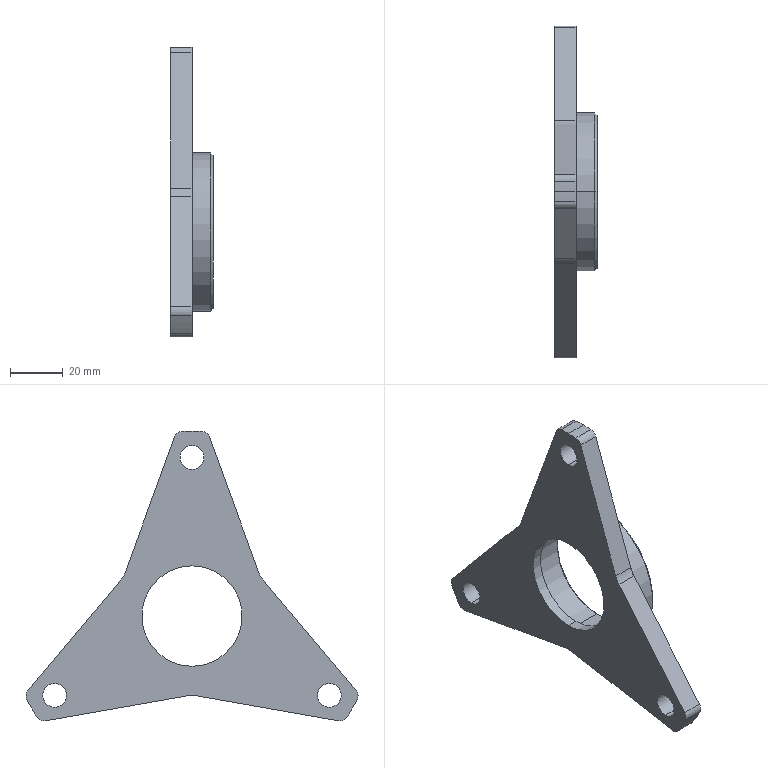Part | SolidWorks | features BaseBody 1 | 1 solid | 41 faces | box 16 x 125.605 x 109.685 mm | volume 50811 mm3 | cylinder 25 | plane 12 | cone 4 | commonest cylinder face diameters 6 x6 9 x6 140 x4 20 x3 38 x2 42 x2
STEP:
#1=CARTESIAN_POINT('',(8.,-51.962,-34.5));
#2=VERTEX_POINT('',#1);
#3=CARTESIAN_POINT('',(8.,-51.962,-25.5));
#4=VERTEX_POINT('',#3);
#5=CARTESIAN_POINT('',(8.,-51.962,-30.));
#6=DIRECTION('',(-1.,0.,0.));
#7=DIRECTION('',(0.,0.,1.));
#8=AXIS2_PLACEMENT_3D('',#5,#6,#7);
#9=CIRCLE('',#8,4.5);
#10=EDGE_CURVE('',#2,#4,#9,.T.);
#11=ORIENTED_EDGE('',*,*,#10,.F.);
#12=CARTESIAN_POINT('',(0.,-51.962,-34.5));
#13=VERTEX_POINT('',#12);
#14=CARTESIAN_POINT('',(0.,-51.962,-34.5));
#15=DIRECTION('',(-1.,0.,0.));
#16=VECTOR('',#15,1000.);
#17=LINE('',#14,#16);
#18=EDGE_CURVE('',#2,#13,#17,.T.);
#19=ORIENTED_EDGE('',*,*,#18,.T.);
#20=CARTESIAN_POINT('',(0.,-51.962,-25.5));
#21=VERTEX_POINT('',#20);
#22=CARTESIAN_POINT('',(0.,-51.962,-30.));
#23=DIRECTION('',(-1.,0.,0.));
#24=DIRECTION('',(0.,0.,1.));
#25=AXIS2_PLACEMENT_3D('',#22,#23,#24);
#26=CIRCLE('',#25,4.5);
#27=EDGE_CURVE('',#13,#21,#26,.T.);
#28=ORIENTED_EDGE('',*,*,#27,.T.);
#29=CARTESIAN_POINT('',(0.,-51.962,-25.5));
#30=DIRECTION('',(-1.,0.,0.));
#31=VECTOR('',#30,1000.);
#32=LINE('',#29,#31);
#33=EDGE_CURVE('',#4,#21,#32,.T.);
#34=ORIENTED_EDGE('',*,*,#33,.F.);
#35=EDGE_LOOP('',(#11,#19,#28,#34));
#36=FACE_OUTER_BOUND('',#35,.T.);
#37=CARTESIAN_POINT('',(0.,-51.962,-30.));
#38=DIRECTION('',(-1.,0.,0.));
#39=DIRECTION('',(0.,0.,1.));
#40=AXIS2_PLACEMENT_3D('',#37,#38,#39);
#41=CYLINDRICAL_SURFACE('',#40,4.5);
#42=ADVANCED_FACE('',(#36),#41,.F.);
#43=CARTESIAN_POINT('',(8.,-3.905,69.891));
#44=VERTEX_POINT('',#43);
#45=CARTESIAN_POINT('',(8.,0.,70.));
#46=VERTEX_POINT('',#45);
#47=CARTESIAN_POINT('',(8.,0.,0.));
#48=DIRECTION('',(-1.,0.,0.));
#49=DIRECTION('',(0.,0.,1.));
#50=AXIS2_PLACEMENT_3D('',#47,#48,#49);
#51=CIRCLE('',#50,70.);
#52=EDGE_CURVE('',#44,#46,#51,.T.);
#53=ORIENTED_EDGE('',*,*,#52,.T.);
#54=CARTESIAN_POINT('',(0.,0.,70.));
#55=VERTEX_POINT('',#54);
#56=CARTESIAN_POINT('',(0.,0.,70.));
#57=DIRECTION('',(-1.,0.,0.));
#58=VECTOR('',#57,1000.);
#59=LINE('',#56,#58);
#60=EDGE_CURVE('',#46,#55,#59,.T.);
#61=ORIENTED_EDGE('',*,*,#60,.T.);
#62=CARTESIAN_POINT('',(0.,-3.905,69.891));
#63=VERTEX_POINT('',#62);
#64=CARTESIAN_POINT('',(0.,0.,0.));
#65=DIRECTION('',(1.,0.,0.));
#66=DIRECTION('',(0.,0.,1.));
#67=AXIS2_PLACEMENT_3D('',#64,#65,#66);
#68=CIRCLE('',#67,70.);
#69=EDGE_CURVE('',#55,#63,#68,.T.);
#70=ORIENTED_EDGE('',*,*,#69,.T.);
#71=CARTESIAN_POINT('',(0.,-3.905,69.891));
#72=DIRECTION('',(-1.,0.,0.));
#73=VECTOR('',#72,1000.);
#74=LINE('',#71,#73);
#75=EDGE_CURVE('',#44,#63,#74,.T.);
#76=ORIENTED_EDGE('',*,*,#75,.F.);
#77=EDGE_LOOP('',(#53,#61,#70,#76));
#78=FACE_OUTER_BOUND('',#77,.T.);
#79=CARTESIAN_POINT('',(0.,0.,0.));
#80=DIRECTION('',(-1.,0.,0.));
#81=DIRECTION('',(0.,0.,1.));
#82=AXIS2_PLACEMENT_3D('',#79,#80,#81);
#83=CYLINDRICAL_SURFACE('',#82,70.);
#84=ADVANCED_FACE('',(#78),#83,.T.);
#85=CARTESIAN_POINT('',(4.,0.,-19.));
#86=VERTEX_POINT('',#85);
#87=CARTESIAN_POINT('',(4.,0.,19.));
#88=VERTEX_POINT('',#87);
#89=CARTESIAN_POINT('',(4.,0.,0.));
#90=DIRECTION('',(-1.,0.,0.));
#91=DIRECTION('',(0.,0.,1.));
#92=AXIS2_PLACEMENT_3D('',#89,#90,#91);
#93=CIRCLE('',#92,19.);
#94=EDGE_CURVE('',#86,#88,#93,.T.);
#95=ORIENTED_EDGE('',*,*,#94,.F.);
#96=CARTESIAN_POINT('',(0.,0.,-19.));
#97=VERTEX_POINT('',#96);
#98=CARTESIAN_POINT('',(0.,0.,-19.));
#99=DIRECTION('',(-1.,0.,0.));
#100=VECTOR('',#99,1000.);
#101=LINE('',#98,#100);
#102=EDGE_CURVE('',#86,#97,#101,.T.);
#103=ORIENTED_EDGE('',*,*,#102,.T.);
#104=CARTESIAN_POINT('',(0.,0.,19.));
#105=VERTEX_POINT('',#104);
#106=CARTESIAN_POINT('',(0.,0.,0.));
#107=DIRECTION('',(-1.,0.,0.));
#108=DIRECTION('',(0.,0.,1.));
#109=AXIS2_PLACEMENT_3D('',#106,#107,#108);
#110=CIRCLE('',#109,19.);
#111=EDGE_CURVE('',#97,#105,#110,.T.);
#112=ORIENTED_EDGE('',*,*,#111,.T.);
#113=CARTESIAN_POINT('',(0.,0.,19.));
#114=DIRECTION('',(-1.,0.,0.));
#115=VECTOR('',#114,1000.);
#116=LINE('',#113,#115);
#117=EDGE_CURVE('',#88,#105,#116,.T.);
#118=ORIENTED_EDGE('',*,*,#117,.F.);
#119=EDGE_LOOP('',(#95,#103,#112,#118));
#120=FACE_OUTER_BOUND('',#119,.T.);
#121=CARTESIAN_POINT('',(0.,0.,0.));
#122=DIRECTION('',(-1.,0.,0.));
#123=DIRECTION('',(0.,0.,1.));
#124=AXIS2_PLACEMENT_3D('',#121,#122,#123);
#125=CYLINDRICAL_SURFACE('',#124,19.);
#126=ADVANCED_FACE('',(#120),#125,.F.);
#127=CARTESIAN_POINT('',(8.,0.,55.5));
#128=VERTEX_POINT('',#127);
#129=CARTESIAN_POINT('',(8.,0.,64.5));
#130=VERTEX_POINT('',#129);
#131=CARTESIAN_POINT('',(8.,0.,60.));
#132=DIRECTION('',(-1.,0.,0.));
#133=DIRECTION('',(0.,0.,1.));
#134=AXIS2_PLACEMENT_3D('',#131,#132,#133);
#135=CIRCLE('',#134,4.5);
#136=EDGE_CURVE('',#128,#130,#135,.T.);
#137=ORIENTED_EDGE('',*,*,#136,.F.);
#138=CARTESIAN_POINT('',(0.,0.,55.5));
#139=VERTEX_POINT('',#138);
#140=CARTESIAN_POINT('',(0.,0.,55.5));
#141=DIRECTION('',(-1.,0.,0.));
#142=VECTOR('',#141,1000.);
#143=LINE('',#140,#142);
#144=EDGE_CURVE('',#128,#139,#143,.T.);
#145=ORIENTED_EDGE('',*,*,#144,.T.);
#146=CARTESIAN_POINT('',(0.,0.,64.5));
#147=VERTEX_POINT('',#146);
#148=CARTESIAN_POINT('',(0.,0.,60.));
#149=DIRECTION('',(-1.,0.,0.));
#150=DIRECTION('',(0.,0.,1.));
#151=AXIS2_PLACEMENT_3D('',#148,#149,#150);
#152=CIRCLE('',#151,4.5);
#153=EDGE_CURVE('',#139,#147,#152,.T.);
#154=ORIENTED_EDGE('',*,*,#153,.T.);
#155=CARTESIAN_POINT('',(0.,0.,64.5));
#156=DIRECTION('',(-1.,0.,0.));
#157=VECTOR('',#156,1000.);
#158=LINE('',#155,#157);
#159=EDGE_CURVE('',#130,#147,#158,.T.);
#160=ORIENTED_EDGE('',*,*,#159,.F.);
#161=EDGE_LOOP('',(#137,#145,#154,#160));
#162=FACE_OUTER_BOUND('',#161,.T.);
#163=CARTESIAN_POINT('',(0.,0.,60.));
#164=DIRECTION('',(-1.,0.,0.));
#165=DIRECTION('',(0.,0.,1.));
#166=AXIS2_PLACEMENT_3D('',#163,#164,#165);
#167=CYLINDRICAL_SURFACE('',#166,4.5);
#168=ADVANCED_FACE('',(#162),#167,.F.);
#169=CARTESIAN_POINT('',(8.,51.962,-34.5));
#170=VERTEX_POINT('',#169);
#171=CARTESIAN_POINT('',(8.,51.962,-25.5));
#172=VERTEX_POINT('',#171);
#173=CARTESIAN_POINT('',(8.,51.962,-30.));
#174=DIRECTION('',(-1.,0.,0.));
#175=DIRECTION('',(0.,0.,1.));
#176=AXIS2_PLACEMENT_3D('',#173,#174,#175);
#177=CIRCLE('',#176,4.5);
#178=EDGE_CURVE('',#170,#172,#177,.T.);
#179=ORIENTED_EDGE('',*,*,#178,.F.);
#180=CARTESIAN_POINT('',(0.,51.962,-34.5));
#181=VERTEX_POINT('',#180);
#182=CARTESIAN_POINT('',(0.,51.962,-34.5));
#183=DIRECTION('',(-1.,0.,0.));
#184=VECTOR('',#183,1000.);
#185=LINE('',#182,#184);
#186=EDGE_CURVE('',#170,#181,#185,.T.);
#187=ORIENTED_EDGE('',*,*,#186,.T.);
#188=CARTESIAN_POINT('',(0.,51.962,-25.5));
#189=VERTEX_POINT('',#188);
#190=CARTESIAN_POINT('',(0.,51.962,-30.));
#191=DIRECTION('',(-1.,0.,0.));
#192=DIRECTION('',(0.,0.,1.));
#193=AXIS2_PLACEMENT_3D('',#190,#191,#192);
#194=CIRCLE('',#193,4.5);
#195=EDGE_CURVE('',#181,#189,#194,.T.);
#196=ORIENTED_EDGE('',*,*,#195,.T.);
#197=CARTESIAN_POINT('',(0.,51.962,-25.5));
#198=DIRECTION('',(-1.,0.,0.));
#199=VECTOR('',#198,1000.);
#200=LINE('',#197,#199);
#201=EDGE_CURVE('',#172,#189,#200,.T.);
#202=ORIENTED_EDGE('',*,*,#201,.F.);
#203=EDGE_LOOP('',(#179,#187,#196,#202));
#204=FACE_OUTER_BOUND('',#203,.T.);
#205=CARTESIAN_POINT('',(0.,51.962,-30.));
#206=DIRECTION('',(-1.,0.,0.));
#207=DIRECTION('',(0.,0.,1.));
#208=AXIS2_PLACEMENT_3D('',#205,#206,#207);
#209=CYLINDRICAL_SURFACE('',#208,4.5);
#210=ADVANCED_FACE('',(#204),#209,.F.);
#211=CARTESIAN_POINT('',(15.,0.,30.));
#212=VERTEX_POINT('',#211);
#213=CARTESIAN_POINT('',(15.,0.,-30.));
#214=VERTEX_POINT('',#213);
#215=CARTESIAN_POINT('',(15.,0.,0.));
#216=DIRECTION('',(-1.,0.,0.));
#217=DIRECTION('',(0.,0.,1.));
#218=AXIS2_PLACEMENT_3D('',#215,#216,#217);
#219=CIRCLE('',#218,30.);
#220=EDGE_CURVE('',#212,#214,#219,.T.);
#221=ORIENTED_EDGE('',*,*,#220,.T.);
#222=CARTESIAN_POINT('',(8.,0.,-30.));
#223=VERTEX_POINT('',#222);
#224=CARTESIAN_POINT('',(0.,0.,-30.));
#225=DIRECTION('',(-1.,0.,0.));
#226=VECTOR('',#225,1000.);
#227=LINE('',#224,#226);
#228=EDGE_CURVE('',#214,#223,#227,.T.);
#229=ORIENTED_EDGE('',*,*,#228,.T.);
#230=CARTESIAN_POINT('',(8.,25.981,15.));
#231=VERTEX_POINT('',#230);
#232=CARTESIAN_POINT('',(8.,0.,0.));
#233=DIRECTION('',(1.,0.,0.));
#234=DIRECTION('',(0.,0.,1.));
#235=AXIS2_PLACEMENT_3D('',#232,#233,#234);
#236=CIRCLE('',#235,30.);
#237=EDGE_CURVE('',#223,#231,#236,.T.);
#238=ORIENTED_EDGE('',*,*,#237,.T.);
#239=CARTESIAN_POINT('',(8.,0.,30.));
#240=VERTEX_POINT('',#239);
#241=CARTESIAN_POINT('',(8.,0.,0.));
#242=DIRECTION('',(1.,0.,0.));
#243=DIRECTION('',(0.,0.,1.));
#244=AXIS2_PLACEMENT_3D('',#241,#242,#243);
#245=CIRCLE('',#244,30.);
#246=EDGE_CURVE('',#231,#240,#245,.T.);
#247=ORIENTED_EDGE('',*,*,#246,.T.);
#248=CARTESIAN_POINT('',(0.,0.,30.));
#249=DIRECTION('',(-1.,0.,0.));
#250=VECTOR('',#249,1000.);
#251=LINE('',#248,#250);
#252=EDGE_CURVE('',#212,#240,#251,.T.);
#253=ORIENTED_EDGE('',*,*,#252,.F.);
#254=EDGE_LOOP('',(#221,#229,#238,#247,#253));
#255=FACE_OUTER_BOUND('',#254,.T.);
#256=CARTESIAN_POINT('',(0.,0.,0.));
#257=DIRECTION('',(-1.,0.,0.));
#258=DIRECTION('',(0.,0.,1.));
#259=AXIS2_PLACEMENT_3D('',#256,#257,#258);
#260=CYLINDRICAL_SURFACE('',#259,30.);
#261=ADVANCED_FACE('',(#255),#260,.T.);
#262=CARTESIAN_POINT('',(15.,0.,-21.));
#263=VERTEX_POINT('',#262);
#264=CARTESIAN_POINT('',(15.,0.,21.));
#265=VERTEX_POINT('',#264);
#266=CARTESIAN_POINT('',(15.,0.,0.));
#267=DIRECTION('',(-1.,0.,0.));
#268=DIRECTION('',(0.,0.,1.));
#269=AXIS2_PLACEMENT_3D('',#266,#267,#268);
#270=CIRCLE('',#269,21.);
#271=EDGE_CURVE('',#263,#265,#270,.T.);
#272=ORIENTED_EDGE('',*,*,#271,.F.);
#273=CARTESIAN_POINT('',(4.,0.,-21.));
#274=VERTEX_POINT('',#273);
#275=CARTESIAN_POINT('',(0.,0.,-21.));
#276=DIRECTION('',(-1.,0.,0.));
#277=VECTOR('',#276,1000.);
#278=LINE('',#275,#277);
#279=EDGE_CURVE('',#263,#274,#278,.T.);
#280=ORIENTED_EDGE('',*,*,#279,.T.);
#281=CARTESIAN_POINT('',(4.,0.,21.));
#282=VERTEX_POINT('',#281);
#283=CARTESIAN_POINT('',(4.,0.,0.));
#284=DIRECTION('',(-1.,0.,0.));
#285=DIRECTION('',(0.,0.,1.));
#286=AXIS2_PLACEMENT_3D('',#283,#284,#285);
#287=CIRCLE('',#286,21.);
#288=EDGE_CURVE('',#274,#282,#287,.T.);
#289=ORIENTED_EDGE('',*,*,#288,.T.);
#290=CARTESIAN_POINT('',(0.,0.,21.));
#291=DIRECTION('',(-1.,0.,0.));
#292=VECTOR('',#291,1000.);
#293=LINE('',#290,#292);
#294=EDGE_CURVE('',#265,#282,#293,.T.);
#295=ORIENTED_EDGE('',*,*,#294,.F.);
#296=EDGE_LOOP('',(#272,#280,#289,#295));
#297=FACE_OUTER_BOUND('',#296,.T.);
#298=CARTESIAN_POINT('',(0.,0.,0.));
#299=DIRECTION('',(-1.,0.,0.));
#300=DIRECTION('',(0.,0.,1.));
#301=AXIS2_PLACEMENT_3D('',#298,#299,#300);
#302=CYLINDRICAL_SURFACE('',#301,21.);
#303=ADVANCED_FACE('',(#297),#302,.F.);
#304=CARTESIAN_POINT('',(16.,0.,29.));
#305=VERTEX_POINT('',#304);
#306=CARTESIAN_POINT('',(16.,0.,-29.));
#307=VERTEX_POINT('',#306);
#308=CARTESIAN_POINT('',(16.,0.,0.));
#309=DIRECTION('',(-1.,0.,0.));
#310=DIRECTION('',(0.,0.,1.));
#311=AXIS2_PLACEMENT_3D('',#308,#309,#310);
#312=CIRCLE('',#311,29.);
#313=EDGE_CURVE('',#305,#307,#312,.T.);
#314=ORIENTED_EDGE('',*,*,#313,.T.);
#315=CARTESIAN_POINT('',(15.,0.,-30.));
#316=DIRECTION('',(-0.7071,0.,-0.7071));
#317=VECTOR('',#316,1000.);
#318=LINE('',#315,#317);
#319=EDGE_CURVE('',#307,#214,#318,.T.);
#320=ORIENTED_EDGE('',*,*,#319,.T.);
#321=ORIENTED_EDGE('',*,*,#220,.F.);
#322=CARTESIAN_POINT('',(15.,0.,30.));
#323=DIRECTION('',(-0.7071,0.,0.7071));
#324=VECTOR('',#323,1000.);
#325=LINE('',#322,#324);
#326=EDGE_CURVE('',#305,#212,#325,.T.);
#327=ORIENTED_EDGE('',*,*,#326,.F.);
#328=EDGE_LOOP('',(#314,#320,#321,#327));
#329=FACE_OUTER_BOUND('',#328,.T.);
#330=CARTESIAN_POINT('',(15.,0.,0.));
#331=DIRECTION('',(-1.,0.,0.));
#332=DIRECTION('',(0.,0.,1.));
#333=AXIS2_PLACEMENT_3D('',#330,#331,#332);
#334=CONICAL_SURFACE('',#333,30.,0.7854);
#335=ADVANCED_FACE('',(#329),#334,.T.);
#336=ORIENTED_EDGE('',*,*,#271,.T.);
#337=CARTESIAN_POINT('',(16.,0.,22.));
#338=VERTEX_POINT('',#337);
#339=CARTESIAN_POINT('',(16.,0.,22.));
#340=DIRECTION('',(0.7071,0.,0.7071));
#341=VECTOR('',#340,1000.);
#342=LINE('',#339,#341);
#343=EDGE_CURVE('',#265,#338,#342,.T.);
#344=ORIENTED_EDGE('',*,*,#343,.T.);
#345=CARTESIAN_POINT('',(16.,0.,-22.));
#346=VERTEX_POINT('',#345);
#347=CARTESIAN_POINT('',(16.,0.,0.));
#348=DIRECTION('',(-1.,0.,0.));
#349=DIRECTION('',(0.,0.,-1.));
#350=AXIS2_PLACEMENT_3D('',#347,#348,#349);
#351=CIRCLE('',#350,22.);
#352=EDGE_CURVE('',#346,#338,#351,.T.);
#353=ORIENTED_EDGE('',*,*,#352,.F.);
#354=CARTESIAN_POINT('',(16.,0.,-22.));
#355=DIRECTION('',(0.7071,0.,-0.7071));
#356=VECTOR('',#355,1000.);
#357=LINE('',#354,#356);
#358=EDGE_CURVE('',#263,#346,#357,.T.);
#359=ORIENTED_EDGE('',*,*,#358,.F.);
#360=EDGE_LOOP('',(#336,#344,#353,#359));
#361=FACE_OUTER_BOUND('',#360,.T.);
#362=CARTESIAN_POINT('',(16.,0.,0.));
#363=DIRECTION('',(1.,0.,0.));
#364=DIRECTION('',(0.,0.,-1.));
#365=AXIS2_PLACEMENT_3D('',#362,#363,#364);
#366=CONICAL_SURFACE('',#365,22.,0.7854);
#367=ADVANCED_FACE('',(#361),#366,.F.);
#368=CARTESIAN_POINT('',(0.,-51.962,-30.));
#369=DIRECTION('',(-1.,0.,0.));
#370=DIRECTION('',(0.,0.,1.));
#371=AXIS2_PLACEMENT_3D('',#368,#369,#370);
#372=CIRCLE('',#371,4.5);
#373=EDGE_CURVE('',#21,#13,#372,.T.);
#374=ORIENTED_EDGE('',*,*,#373,.F.);
#375=ORIENTED_EDGE('',*,*,#27,.F.);
#376=EDGE_LOOP('',(#374,#375));
#377=FACE_BOUND('',#376,.T.);
#378=CARTESIAN_POINT('',(0.,-58.575,-38.328));
#379=VERTEX_POINT('',#378);
#380=CARTESIAN_POINT('',(0.,-55.543,-39.64));
#381=VERTEX_POINT('',#380);
#382=CARTESIAN_POINT('',(0.,-56.064,-36.685));
#383=DIRECTION('',(1.,0.,0.));
#384=DIRECTION('',(0.,0.,1.));
#385=AXIS2_PLACEMENT_3D('',#382,#383,#384);
#386=CIRCLE('',#385,3.);
#387=EDGE_CURVE('',#379,#381,#386,.T.);
#388=ORIENTED_EDGE('',*,*,#387,.F.);
#389=CARTESIAN_POINT('',(0.,-62.48,-31.563));
#390=VERTEX_POINT('',#389);
#391=CARTESIAN_POINT('',(0.,0.,0.));
#392=DIRECTION('',(1.,0.,0.));
#393=DIRECTION('',(0.,0.,1.));
#394=AXIS2_PLACEMENT_3D('',#391,#392,#393);
#395=CIRCLE('',#394,70.);
#396=EDGE_CURVE('',#390,#379,#395,.T.);
#397=ORIENTED_EDGE('',*,*,#396,.F.);
#398=CARTESIAN_POINT('',(0.,-62.101,-28.282));
#399=VERTEX_POINT('',#398);
#400=CARTESIAN_POINT('',(0.,-59.802,-30.211));
#401=DIRECTION('',(1.,0.,0.));
#402=DIRECTION('',(0.,0.,1.));
#403=AXIS2_PLACEMENT_3D('',#400,#401,#402);
#404=CIRCLE('',#403,3.);
#405=EDGE_CURVE('',#399,#390,#404,.T.);
#406=ORIENTED_EDGE('',*,*,#405,.F.);
#407=CARTESIAN_POINT('',(0.,-26.981,13.572));
#408=VERTEX_POINT('',#407);
#409=CARTESIAN_POINT('',(0.,-26.981,13.572));
#410=DIRECTION('',(0.,-0.6428,-0.766));
#411=VECTOR('',#410,1000.);
#412=LINE('',#409,#411);
#413=EDGE_CURVE('',#408,#399,#412,.T.);
#414=ORIENTED_EDGE('',*,*,#413,.F.);
#415=CARTESIAN_POINT('',(0.,-25.244,16.58));
#416=VERTEX_POINT('',#415);
#417=CARTESIAN_POINT('',(0.,-34.641,20.));
#418=DIRECTION('',(-1.,0.,0.));
#419=DIRECTION('',(0.,0.,-1.));
#420=AXIS2_PLACEMENT_3D('',#417,#418,#419);
#421=CIRCLE('',#420,10.);
#422=EDGE_CURVE('',#416,#408,#421,.T.);
#423=ORIENTED_EDGE('',*,*,#422,.F.);
#424=CARTESIAN_POINT('',(0.,-6.557,67.922));
#425=VERTEX_POINT('',#424);
#426=CARTESIAN_POINT('',(0.,-6.557,67.922));
#427=DIRECTION('',(0.,-0.342,-0.9397));
#428=VECTOR('',#427,1000.);
#429=LINE('',#426,#428);
#430=EDGE_CURVE('',#425,#416,#429,.T.);
#431=ORIENTED_EDGE('',*,*,#430,.F.);
#432=CARTESIAN_POINT('',(0.,-3.738,66.896));
#433=DIRECTION('',(1.,0.,0.));
#434=DIRECTION('',(0.,0.,1.));
#435=AXIS2_PLACEMENT_3D('',#432,#433,#434);
#436=CIRCLE('',#435,3.);
#437=EDGE_CURVE('',#63,#425,#436,.T.);
#438=ORIENTED_EDGE('',*,*,#437,.F.);
#439=ORIENTED_EDGE('',*,*,#69,.F.);
#440=CARTESIAN_POINT('',(0.,3.905,69.891));
#441=VERTEX_POINT('',#440);
#442=CARTESIAN_POINT('',(0.,0.,0.));
#443=DIRECTION('',(1.,0.,0.));
#444=DIRECTION('',(0.,0.,1.));
#445=AXIS2_PLACEMENT_3D('',#442,#443,#444);
#446=CIRCLE('',#445,70.);
#447=EDGE_CURVE('',#441,#55,#446,.T.);
#448=ORIENTED_EDGE('',*,*,#447,.F.);
#449=CARTESIAN_POINT('',(0.,6.557,67.922));
#450=VERTEX_POINT('',#449);
#451=CARTESIAN_POINT('',(0.,3.738,66.896));
#452=DIRECTION('',(1.,0.,0.));
#453=DIRECTION('',(0.,0.,1.));
#454=AXIS2_PLACEMENT_3D('',#451,#452,#453);
#455=CIRCLE('',#454,3.);
#456=EDGE_CURVE('',#450,#441,#455,.T.);
#457=ORIENTED_EDGE('',*,*,#456,.F.);
#458=CARTESIAN_POINT('',(0.,25.244,16.58));
#459=VERTEX_POINT('',#458);
#460=CARTESIAN_POINT('',(0.,25.244,16.58));
#461=DIRECTION('',(0.,-0.342,0.9397));
#462=VECTOR('',#461,1000.);
#463=LINE('',#460,#462);
#464=EDGE_CURVE('',#459,#450,#463,.T.);
#465=ORIENTED_EDGE('',*,*,#464,.F.);
#466=CARTESIAN_POINT('',(0.,26.981,13.572));
#467=VERTEX_POINT('',#466);
#468=CARTESIAN_POINT('',(0.,34.641,20.));
#469=DIRECTION('',(-1.,0.,0.));
#470=DIRECTION('',(0.,0.,-1.));
#471=AXIS2_PLACEMENT_3D('',#468,#469,#470);
#472=CIRCLE('',#471,10.);
#473=EDGE_CURVE('',#467,#459,#472,.T.);
#474=ORIENTED_EDGE('',*,*,#473,.F.);
#475=CARTESIAN_POINT('',(0.,62.101,-28.282));
#476=VERTEX_POINT('',#475);
#477=CARTESIAN_POINT('',(0.,62.101,-28.282));
#478=DIRECTION('',(0.,-0.6428,0.766));
#479=VECTOR('',#478,1000.);
#480=LINE('',#477,#479);
#481=EDGE_CURVE('',#476,#467,#480,.T.);
#482=ORIENTED_EDGE('',*,*,#481,.F.);
#483=CARTESIAN_POINT('',(0.,62.48,-31.563));
#484=VERTEX_POINT('',#483);
#485=CARTESIAN_POINT('',(0.,59.802,-30.211));
#486=DIRECTION('',(1.,0.,0.));
#487=DIRECTION('',(0.,0.,1.));
#488=AXIS2_PLACEMENT_3D('',#485,#486,#487);
#489=CIRCLE('',#488,3.);
#490=EDGE_CURVE('',#484,#476,#489,.T.);
#491=ORIENTED_EDGE('',*,*,#490,.F.);
#492=CARTESIAN_POINT('',(0.,58.575,-38.328));
#493=VERTEX_POINT('',#492);
#494=CARTESIAN_POINT('',(0.,0.,0.));
#495=DIRECTION('',(1.,0.,0.));
#496=DIRECTION('',(0.,0.,1.));
#497=AXIS2_PLACEMENT_3D('',#494,#495,#496);
#498=CIRCLE('',#497,70.);
#499=EDGE_CURVE('',#493,#484,#498,.T.);
#500=ORIENTED_EDGE('',*,*,#499,.F.);
#501=CARTESIAN_POINT('',(0.,55.543,-39.64));
#502=VERTEX_POINT('',#501);
#503=CARTESIAN_POINT('',(0.,56.064,-36.685));
#504=DIRECTION('',(1.,0.,0.));
#505=DIRECTION('',(0.,0.,1.));
#506=AXIS2_PLACEMENT_3D('',#503,#504,#505);
#507=CIRCLE('',#506,3.);
#508=EDGE_CURVE('',#502,#493,#507,.T.);
#509=ORIENTED_EDGE('',*,*,#508,.F.);
#510=CARTESIAN_POINT('',(0.,1.736,-30.152));
#511=VERTEX_POINT('',#510);
#512=CARTESIAN_POINT('',(0.,1.736,-30.152));
#513=DIRECTION('',(0.,0.9848,-0.1736));
#514=VECTOR('',#513,1000.);
#515=LINE('',#512,#514);
#516=EDGE_CURVE('',#511,#502,#515,.T.);
#517=ORIENTED_EDGE('',*,*,#516,.F.);
#518=CARTESIAN_POINT('',(0.,-1.736,-30.152));
#519=VERTEX_POINT('',#518);
#520=CARTESIAN_POINT('',(0.,0.,-40.));
#521=DIRECTION('',(-1.,0.,0.));
#522=DIRECTION('',(0.,0.,-1.));
#523=AXIS2_PLACEMENT_3D('',#520,#521,#522);
#524=CIRCLE('',#523,10.);
#525=EDGE_CURVE('',#519,#511,#524,.T.);
#526=ORIENTED_EDGE('',*,*,#525,.F.);
#527=CARTESIAN_POINT('',(0.,-55.543,-39.64));
#528=DIRECTION('',(0.,0.9848,0.1736));
#529=VECTOR('',#528,1000.);
#530=LINE('',#527,#529);
#531=EDGE_CURVE('',#381,#519,#530,.T.);
#532=ORIENTED_EDGE('',*,*,#531,.F.);
#533=EDGE_LOOP('',(#388,#397,#406,#414,#423,#431,#438,#439,#448,#457,#465,#474,#482,#491,#500,#509,#517,#526,#532));
#534=FACE_OUTER_BOUND('',#533,.T.);
#535=CARTESIAN_POINT('',(0.,0.,0.));
#536=DIRECTION('',(-1.,0.,0.));
#537=DIRECTION('',(0.,0.,1.));
#538=AXIS2_PLACEMENT_3D('',#535,#536,#537);
#539=CIRCLE('',#538,19.);
#540=EDGE_CURVE('',#105,#97,#539,.T.);
#541=ORIENTED_EDGE('',*,*,#540,.F.);
#542=ORIENTED_EDGE('',*,*,#111,.F.);
#543=EDGE_LOOP('',(#541,#542));
#544=FACE_BOUND('',#543,.T.);
#545=CARTESIAN_POINT('',(0.,0.,60.));
#546=DIRECTION('',(-1.,0.,0.));
#547=DIRECTION('',(0.,0.,1.));
#548=AXIS2_PLACEMENT_3D('',#545,#546,#547);
#549=CIRCLE('',#548,4.5);
#550=EDGE_CURVE('',#147,#139,#549,.T.);
#551=ORIENTED_EDGE('',*,*,#550,.F.);
#552=ORIENTED_EDGE('',*,*,#153,.F.);
#553=EDGE_LOOP('',(#551,#552));
#554=FACE_BOUND('',#553,.T.);
#555=CARTESIAN_POINT('',(0.,51.962,-30.));
#556=DIRECTION('',(-1.,0.,0.));
#557=DIRECTION('',(0.,0.,1.));
#558=AXIS2_PLACEMENT_3D('',#555,#556,#557);
#559=CIRCLE('',#558,4.5);
#560=EDGE_CURVE('',#189,#181,#559,.T.);
#561=ORIENTED_EDGE('',*,*,#560,.F.);
#562=ORIENTED_EDGE('',*,*,#195,.F.);
#563=EDGE_LOOP('',(#561,#562));
#564=FACE_BOUND('',#563,.T.);
#565=CARTESIAN_POINT('',(0.,19.,0.));
#566=DIRECTION('',(1.,0.,0.));
#567=DIRECTION('',(0.,0.,-1.));
#568=AXIS2_PLACEMENT_3D('',#565,#566,#567);
#569=PLANE('',#568);
#570=ADVANCED_FACE('',(#377,#534,#544,#554,#564),#569,.F.);
#571=ORIENTED_EDGE('',*,*,#18,.F.);
#572=CARTESIAN_POINT('',(8.,-51.962,-30.));
#573=DIRECTION('',(-1.,0.,0.));
#574=DIRECTION('',(0.,0.,1.));
#575=AXIS2_PLACEMENT_3D('',#572,#573,#574);
#576=CIRCLE('',#575,4.5);
#577=EDGE_CURVE('',#4,#2,#576,.T.);
#578=ORIENTED_EDGE('',*,*,#577,.F.);
#579=ORIENTED_EDGE('',*,*,#33,.T.);
#580=ORIENTED_EDGE('',*,*,#373,.T.);
#581=EDGE_LOOP('',(#571,#578,#579,#580));
#582=FACE_OUTER_BOUND('',#581,.T.);
#583=CARTESIAN_POINT('',(0.,-51.962,-30.));
#584=DIRECTION('',(-1.,0.,0.));
#585=DIRECTION('',(0.,0.,1.));
#586=AXIS2_PLACEMENT_3D('',#583,#584,#585);
#587=CYLINDRICAL_SURFACE('',#586,4.5);
#588=ADVANCED_FACE('',(#582),#587,.F.);
#589=ORIENTED_EDGE('',*,*,#531,.T.);
#590=CARTESIAN_POINT('',(8.,-1.736,-30.152));
#591=VERTEX_POINT('',#590);
#592=CARTESIAN_POINT('',(-253.294,-1.736,-30.152));
#593=DIRECTION('',(1.,0.,0.));
#594=VECTOR('',#593,1000.);
#595=LINE('',#592,#594);
#596=EDGE_CURVE('',#519,#591,#595,.T.);
#597=ORIENTED_EDGE('',*,*,#596,.T.);
#598=CARTESIAN_POINT('',(8.,-55.543,-39.64));
#599=VERTEX_POINT('',#598);
#600=CARTESIAN_POINT('',(8.,-57.461,-39.978));
#601=DIRECTION('',(0.,-0.9848,-0.1736));
#602=VECTOR('',#601,1000.);
#603=LINE('',#600,#602);
#604=EDGE_CURVE('',#591,#599,#603,.T.);
#605=ORIENTED_EDGE('',*,*,#604,.T.);
#606=CARTESIAN_POINT('',(-253.294,-55.543,-39.64));
#607=DIRECTION('',(-1.,0.,0.));
#608=VECTOR('',#607,1000.);
#609=LINE('',#606,#608);
#610=EDGE_CURVE('',#599,#381,#609,.T.);
#611=ORIENTED_EDGE('',*,*,#610,.T.);
#612=EDGE_LOOP('',(#589,#597,#605,#611));
#613=FACE_OUTER_BOUND('',#612,.T.);
#614=CARTESIAN_POINT('',(-253.294,-57.461,-39.978));
#615=DIRECTION('',(0.,0.1736,-0.9848));
#616=DIRECTION('',(0.,0.9848,0.1736));
#617=AXIS2_PLACEMENT_3D('',#614,#615,#616);
#618=PLANE('',#617);
#619=ADVANCED_FACE('',(#613),#618,.T.);
#620=CARTESIAN_POINT('',(8.,-58.575,-38.328));
#621=VERTEX_POINT('',#620);
#622=CARTESIAN_POINT('',(8.,-56.064,-36.685));
#623=DIRECTION('',(-1.,0.,0.));
#624=DIRECTION('',(0.,0.,1.));
#625=AXIS2_PLACEMENT_3D('',#622,#623,#624);
#626=CIRCLE('',#625,3.);
#627=EDGE_CURVE('',#599,#621,#626,.T.);
#628=ORIENTED_EDGE('',*,*,#627,.T.);
#629=CARTESIAN_POINT('',(0.,-58.575,-38.328));
#630=DIRECTION('',(-1.,0.,0.));
#631=VECTOR('',#630,1000.);
#632=LINE('',#629,#631);
#633=EDGE_CURVE('',#621,#379,#632,.T.);
#634=ORIENTED_EDGE('',*,*,#633,.T.);
#635=ORIENTED_EDGE('',*,*,#387,.T.);
#636=ORIENTED_EDGE('',*,*,#610,.F.);
#637=EDGE_LOOP('',(#628,#634,#635,#636));
#638=FACE_OUTER_BOUND('',#637,.T.);
#639=CARTESIAN_POINT('',(0.,-56.064,-36.685));
#640=DIRECTION('',(-1.,0.,0.));
#641=DIRECTION('',(0.,0.,1.));
#642=AXIS2_PLACEMENT_3D('',#639,#640,#641);
#643=CYLINDRICAL_SURFACE('',#642,3.);
#644=ADVANCED_FACE('',(#638),#643,.T.);
#645=CARTESIAN_POINT('',(8.,-62.48,-31.563));
#646=VERTEX_POINT('',#645);
#647=CARTESIAN_POINT('',(8.,0.,0.));
#648=DIRECTION('',(-1.,0.,0.));
#649=DIRECTION('',(0.,0.,1.));
#650=AXIS2_PLACEMENT_3D('',#647,#648,#649);
#651=CIRCLE('',#650,70.);
#652=EDGE_CURVE('',#621,#646,#651,.T.);
#653=ORIENTED_EDGE('',*,*,#652,.T.);
#654=CARTESIAN_POINT('',(0.,-62.48,-31.563));
#655=DIRECTION('',(-1.,0.,0.));
#656=VECTOR('',#655,1000.);
#657=LINE('',#654,#656);
#658=EDGE_CURVE('',#646,#390,#657,.T.);
#659=ORIENTED_EDGE('',*,*,#658,.T.);
#660=ORIENTED_EDGE('',*,*,#396,.T.);
#661=ORIENTED_EDGE('',*,*,#633,.F.);
#662=EDGE_LOOP('',(#653,#659,#660,#661));
#663=FACE_OUTER_BOUND('',#662,.T.);
#664=CARTESIAN_POINT('',(0.,0.,0.));
#665=DIRECTION('',(-1.,0.,0.));
#666=DIRECTION('',(0.,0.,1.));
#667=AXIS2_PLACEMENT_3D('',#664,#665,#666);
#668=CYLINDRICAL_SURFACE('',#667,70.);
#669=ADVANCED_FACE('',(#663),#668,.T.);
#670=CARTESIAN_POINT('',(8.,-62.101,-28.282));
#671=VERTEX_POINT('',#670);
#672=CARTESIAN_POINT('',(8.,-59.802,-30.211));
#673=DIRECTION('',(-1.,0.,0.));
#674=DIRECTION('',(0.,0.,1.));
#675=AXIS2_PLACEMENT_3D('',#672,#673,#674);
#676=CIRCLE('',#675,3.);
#677=EDGE_CURVE('',#646,#671,#676,.T.);
#678=ORIENTED_EDGE('',*,*,#677,.T.);
#679=CARTESIAN_POINT('',(0.,-62.101,-28.282));
#680=DIRECTION('',(-1.,0.,0.));
#681=VECTOR('',#680,1000.);
#682=LINE('',#679,#681);
#683=EDGE_CURVE('',#671,#399,#682,.T.);
#684=ORIENTED_EDGE('',*,*,#683,.T.);
#685=ORIENTED_EDGE('',*,*,#405,.T.);
#686=ORIENTED_EDGE('',*,*,#658,.F.);
#687=EDGE_LOOP('',(#678,#684,#685,#686));
#688=FACE_OUTER_BOUND('',#687,.T.);
#689=CARTESIAN_POINT('',(0.,-59.802,-30.211));
#690=DIRECTION('',(-1.,0.,0.));
#691=DIRECTION('',(0.,0.,1.));
#692=AXIS2_PLACEMENT_3D('',#689,#690,#691);
#693=CYLINDRICAL_SURFACE('',#692,3.);
#694=ADVANCED_FACE('',(#688),#693,.T.);
#695=CARTESIAN_POINT('',(8.,-26.981,13.572));
#696=VERTEX_POINT('',#695);
#697=CARTESIAN_POINT('',(8.,-63.352,-29.774));
#698=DIRECTION('',(0.,0.6428,0.766));
#699=VECTOR('',#698,1000.);
#700=LINE('',#697,#699);
#701=EDGE_CURVE('',#671,#696,#700,.T.);
#702=ORIENTED_EDGE('',*,*,#701,.T.);
#703=CARTESIAN_POINT('',(-223.436,-26.981,13.572));
#704=DIRECTION('',(-1.,0.,0.));
#705=VECTOR('',#704,1000.);
#706=LINE('',#703,#705);
#707=EDGE_CURVE('',#696,#408,#706,.T.);
#708=ORIENTED_EDGE('',*,*,#707,.T.);
#709=ORIENTED_EDGE('',*,*,#413,.T.);
#710=ORIENTED_EDGE('',*,*,#683,.F.);
#711=EDGE_LOOP('',(#702,#708,#709,#710));
#712=FACE_OUTER_BOUND('',#711,.T.);
#713=CARTESIAN_POINT('',(-223.436,-63.352,-29.774));
#714=DIRECTION('',(0.,-0.766,0.6428));
#715=DIRECTION('',(0.,-0.6428,-0.766));
#716=AXIS2_PLACEMENT_3D('',#713,#714,#715);
#717=PLANE('',#716);
#718=ADVANCED_FACE('',(#712),#717,.T.);
#719=ORIENTED_EDGE('',*,*,#422,.T.);
#720=ORIENTED_EDGE('',*,*,#707,.F.);
#721=CARTESIAN_POINT('',(8.,-25.981,15.));
#722=VERTEX_POINT('',#721);
#723=CARTESIAN_POINT('',(8.,-34.641,20.));
#724=DIRECTION('',(-1.,0.,0.));
#725=DIRECTION('',(0.,0.,-1.));
#726=AXIS2_PLACEMENT_3D('',#723,#724,#725);
#727=CIRCLE('',#726,10.);
#728=EDGE_CURVE('',#722,#696,#727,.T.);
#729=ORIENTED_EDGE('',*,*,#728,.F.);
#730=CARTESIAN_POINT('',(8.,-25.244,16.58));
#731=VERTEX_POINT('',#730);
#732=CARTESIAN_POINT('',(8.,-34.641,20.));
#733=DIRECTION('',(-1.,0.,0.));
#734=DIRECTION('',(0.,0.,-1.));
#735=AXIS2_PLACEMENT_3D('',#732,#733,#734);
#736=CIRCLE('',#735,10.);
#737=EDGE_CURVE('',#731,#722,#736,.T.);
#738=ORIENTED_EDGE('',*,*,#737,.F.);
#739=CARTESIAN_POINT('',(-223.436,-25.244,16.58));
#740=DIRECTION('',(1.,0.,0.));
#741=VECTOR('',#740,1000.);
#742=LINE('',#739,#741);
#743=EDGE_CURVE('',#416,#731,#742,.T.);
#744=ORIENTED_EDGE('',*,*,#743,.F.);
#745=EDGE_LOOP('',(#719,#720,#729,#738,#744));
#746=FACE_OUTER_BOUND('',#745,.T.);
#747=CARTESIAN_POINT('',(-223.436,-34.641,20.));
#748=DIRECTION('',(1.,0.,0.));
#749=DIRECTION('',(0.,0.,-1.));
#750=AXIS2_PLACEMENT_3D('',#747,#748,#749);
#751=CYLINDRICAL_SURFACE('',#750,10.);
#752=ADVANCED_FACE('',(#746),#751,.F.);
#753=ORIENTED_EDGE('',*,*,#430,.T.);
#754=ORIENTED_EDGE('',*,*,#743,.T.);
#755=CARTESIAN_POINT('',(8.,-6.557,67.922));
#756=VERTEX_POINT('',#755);
#757=CARTESIAN_POINT('',(8.,-5.891,69.752));
#758=DIRECTION('',(0.,0.342,0.9397));
#759=VECTOR('',#758,1000.);
#760=LINE('',#757,#759);
#761=EDGE_CURVE('',#731,#756,#760,.T.);
#762=ORIENTED_EDGE('',*,*,#761,.T.);
#763=CARTESIAN_POINT('',(-223.436,-6.557,67.922));
#764=DIRECTION('',(-1.,0.,0.));
#765=VECTOR('',#764,1000.);
#766=LINE('',#763,#765);
#767=EDGE_CURVE('',#756,#425,#766,.T.);
#768=ORIENTED_EDGE('',*,*,#767,.T.);
#769=EDGE_LOOP('',(#753,#754,#762,#768));
#770=FACE_OUTER_BOUND('',#769,.T.);
#771=CARTESIAN_POINT('',(-223.436,-5.891,69.752));
#772=DIRECTION('',(0.,-0.9397,0.342));
#773=DIRECTION('',(0.,-0.342,-0.9397));
#774=AXIS2_PLACEMENT_3D('',#771,#772,#773);
#775=PLANE('',#774);
#776=ADVANCED_FACE('',(#770),#775,.T.);
#777=CARTESIAN_POINT('',(8.,-3.738,66.896));
#778=DIRECTION('',(-1.,0.,0.));
#779=DIRECTION('',(0.,0.,1.));
#780=AXIS2_PLACEMENT_3D('',#777,#778,#779);
#781=CIRCLE('',#780,3.);
#782=EDGE_CURVE('',#756,#44,#781,.T.);
#783=ORIENTED_EDGE('',*,*,#782,.T.);
#784=ORIENTED_EDGE('',*,*,#75,.T.);
#785=ORIENTED_EDGE('',*,*,#437,.T.);
#786=ORIENTED_EDGE('',*,*,#767,.F.);
#787=EDGE_LOOP('',(#783,#784,#785,#786));
#788=FACE_OUTER_BOUND('',#787,.T.);
#789=CARTESIAN_POINT('',(0.,-3.738,66.896));
#790=DIRECTION('',(-1.,0.,0.));
#791=DIRECTION('',(0.,0.,1.));
#792=AXIS2_PLACEMENT_3D('',#789,#790,#791);
#793=CYLINDRICAL_SURFACE('',#792,3.);
#794=ADVANCED_FACE('',(#788),#793,.T.);
#795=ORIENTED_EDGE('',*,*,#60,.F.);
#796=CARTESIAN_POINT('',(8.,3.905,69.891));
#797=VERTEX_POINT('',#796);
#798=CARTESIAN_POINT('',(8.,0.,0.));
#799=DIRECTION('',(-1.,0.,0.));
#800=DIRECTION('',(0.,0.,1.));
#801=AXIS2_PLACEMENT_3D('',#798,#799,#800);
#802=CIRCLE('',#801,70.);
#803=EDGE_CURVE('',#46,#797,#802,.T.);
#804=ORIENTED_EDGE('',*,*,#803,.T.);
#805=CARTESIAN_POINT('',(0.,3.905,69.891));
#806=DIRECTION('',(-1.,0.,0.));
#807=VECTOR('',#806,1000.);
#808=LINE('',#805,#807);
#809=EDGE_CURVE('',#797,#441,#808,.T.);
#810=ORIENTED_EDGE('',*,*,#809,.T.);
#811=ORIENTED_EDGE('',*,*,#447,.T.);
#812=EDGE_LOOP('',(#795,#804,#810,#811));
#813=FACE_OUTER_BOUND('',#812,.T.);
#814=CARTESIAN_POINT('',(0.,0.,0.));
#815=DIRECTION('',(-1.,0.,0.));
#816=DIRECTION('',(0.,0.,1.));
#817=AXIS2_PLACEMENT_3D('',#814,#815,#816);
#818=CYLINDRICAL_SURFACE('',#817,70.);
#819=ADVANCED_FACE('',(#813),#818,.T.);
#820=CARTESIAN_POINT('',(8.,6.557,67.922));
#821=VERTEX_POINT('',#820);
#822=CARTESIAN_POINT('',(8.,3.738,66.896));
#823=DIRECTION('',(-1.,0.,0.));
#824=DIRECTION('',(0.,0.,1.));
#825=AXIS2_PLACEMENT_3D('',#822,#823,#824);
#826=CIRCLE('',#825,3.);
#827=EDGE_CURVE('',#797,#821,#826,.T.);
#828=ORIENTED_EDGE('',*,*,#827,.T.);
#829=CARTESIAN_POINT('',(0.,6.557,67.922));
#830=DIRECTION('',(-1.,0.,0.));
#831=VECTOR('',#830,1000.);
#832=LINE('',#829,#831);
#833=EDGE_CURVE('',#821,#450,#832,.T.);
#834=ORIENTED_EDGE('',*,*,#833,.T.);
#835=ORIENTED_EDGE('',*,*,#456,.T.);
#836=ORIENTED_EDGE('',*,*,#809,.F.);
#837=EDGE_LOOP('',(#828,#834,#835,#836));
#838=FACE_OUTER_BOUND('',#837,.T.);
#839=CARTESIAN_POINT('',(0.,3.738,66.896));
#840=DIRECTION('',(-1.,0.,0.));
#841=DIRECTION('',(0.,0.,1.));
#842=AXIS2_PLACEMENT_3D('',#839,#840,#841);
#843=CYLINDRICAL_SURFACE('',#842,3.);
#844=ADVANCED_FACE('',(#838),#843,.T.);
#845=CARTESIAN_POINT('',(8.,25.244,16.58));
#846=VERTEX_POINT('',#845);
#847=CARTESIAN_POINT('',(8.,5.891,69.752));
#848=DIRECTION('',(0.,0.342,-0.9397));
#849=VECTOR('',#848,1000.);
#850=LINE('',#847,#849);
#851=EDGE_CURVE('',#821,#846,#850,.T.);
#852=ORIENTED_EDGE('',*,*,#851,.T.);
#853=CARTESIAN_POINT('',(-223.436,25.244,16.58));
#854=DIRECTION('',(-1.,0.,0.));
#855=VECTOR('',#854,1000.);
#856=LINE('',#853,#855);
#857=EDGE_CURVE('',#846,#459,#856,.T.);
#858=ORIENTED_EDGE('',*,*,#857,.T.);
#859=ORIENTED_EDGE('',*,*,#464,.T.);
#860=ORIENTED_EDGE('',*,*,#833,.F.);
#861=EDGE_LOOP('',(#852,#858,#859,#860));
#862=FACE_OUTER_BOUND('',#861,.T.);
#863=CARTESIAN_POINT('',(-223.436,5.891,69.752));
#864=DIRECTION('',(0.,0.9397,0.342));
#865=DIRECTION('',(0.,-0.342,0.9397));
#866=AXIS2_PLACEMENT_3D('',#863,#864,#865);
#867=PLANE('',#866);
#868=ADVANCED_FACE('',(#862),#867,.T.);
#869=ORIENTED_EDGE('',*,*,#473,.T.);
#870=ORIENTED_EDGE('',*,*,#857,.F.);
#871=CARTESIAN_POINT('',(8.,34.641,20.));
#872=DIRECTION('',(-1.,0.,0.));
#873=DIRECTION('',(0.,0.,-1.));
#874=AXIS2_PLACEMENT_3D('',#871,#872,#873);
#875=CIRCLE('',#874,10.);
#876=EDGE_CURVE('',#231,#846,#875,.T.);
#877=ORIENTED_EDGE('',*,*,#876,.F.);
#878=CARTESIAN_POINT('',(8.,26.981,13.572));
#879=VERTEX_POINT('',#878);
#880=CARTESIAN_POINT('',(8.,34.641,20.));
#881=DIRECTION('',(-1.,0.,0.));
#882=DIRECTION('',(0.,0.,-1.));
#883=AXIS2_PLACEMENT_3D('',#880,#881,#882);
#884=CIRCLE('',#883,10.);
#885=EDGE_CURVE('',#879,#231,#884,.T.);
#886=ORIENTED_EDGE('',*,*,#885,.F.);
#887=CARTESIAN_POINT('',(-223.436,26.981,13.572));
#888=DIRECTION('',(1.,0.,0.));
#889=VECTOR('',#888,1000.);
#890=LINE('',#887,#889);
#891=EDGE_CURVE('',#467,#879,#890,.T.);
#892=ORIENTED_EDGE('',*,*,#891,.F.);
#893=EDGE_LOOP('',(#869,#870,#877,#886,#892));
#894=FACE_OUTER_BOUND('',#893,.T.);
#895=CARTESIAN_POINT('',(-223.436,34.641,20.));
#896=DIRECTION('',(1.,0.,0.));
#897=DIRECTION('',(0.,0.,-1.));
#898=AXIS2_PLACEMENT_3D('',#895,#896,#897);
#899=CYLINDRICAL_SURFACE('',#898,10.);
#900=ADVANCED_FACE('',(#894),#899,.F.);
#901=ORIENTED_EDGE('',*,*,#481,.T.);
#902=ORIENTED_EDGE('',*,*,#891,.T.);
#903=CARTESIAN_POINT('',(8.,62.101,-28.282));
#904=VERTEX_POINT('',#903);
#905=CARTESIAN_POINT('',(8.,63.352,-29.774));
#906=DIRECTION('',(0.,0.6428,-0.766));
#907=VECTOR('',#906,1000.);
#908=LINE('',#905,#907);
#909=EDGE_CURVE('',#879,#904,#908,.T.);
#910=ORIENTED_EDGE('',*,*,#909,.T.);
#911=CARTESIAN_POINT('',(-223.436,62.101,-28.282));
#912=DIRECTION('',(-1.,0.,0.));
#913=VECTOR('',#912,1000.);
#914=LINE('',#911,#913);
#915=EDGE_CURVE('',#904,#476,#914,.T.);
#916=ORIENTED_EDGE('',*,*,#915,.T.);
#917=EDGE_LOOP('',(#901,#902,#910,#916));
#918=FACE_OUTER_BOUND('',#917,.T.);
#919=CARTESIAN_POINT('',(-223.436,63.352,-29.774));
#920=DIRECTION('',(0.,0.766,0.6428));
#921=DIRECTION('',(0.,-0.6428,0.766));
#922=AXIS2_PLACEMENT_3D('',#919,#920,#921);
#923=PLANE('',#922);
#924=ADVANCED_FACE('',(#918),#923,.T.);
#925=CARTESIAN_POINT('',(8.,62.48,-31.563));
#926=VERTEX_POINT('',#925);
#927=CARTESIAN_POINT('',(8.,59.802,-30.211));
#928=DIRECTION('',(-1.,0.,0.));
#929=DIRECTION('',(0.,0.,1.));
#930=AXIS2_PLACEMENT_3D('',#927,#928,#929);
#931=CIRCLE('',#930,3.);
#932=EDGE_CURVE('',#904,#926,#931,.T.);
#933=ORIENTED_EDGE('',*,*,#932,.T.);
#934=CARTESIAN_POINT('',(0.,62.48,-31.563));
#935=DIRECTION('',(-1.,0.,0.));
#936=VECTOR('',#935,1000.);
#937=LINE('',#934,#936);
#938=EDGE_CURVE('',#926,#484,#937,.T.);
#939=ORIENTED_EDGE('',*,*,#938,.T.);
#940=ORIENTED_EDGE('',*,*,#490,.T.);
#941=ORIENTED_EDGE('',*,*,#915,.F.);
#942=EDGE_LOOP('',(#933,#939,#940,#941));
#943=FACE_OUTER_BOUND('',#942,.T.);
#944=CARTESIAN_POINT('',(0.,59.802,-30.211));
#945=DIRECTION('',(-1.,0.,0.));
#946=DIRECTION('',(0.,0.,1.));
#947=AXIS2_PLACEMENT_3D('',#944,#945,#946);
#948=CYLINDRICAL_SURFACE('',#947,3.);
#949=ADVANCED_FACE('',(#943),#948,.T.);
#950=CARTESIAN_POINT('',(8.,58.575,-38.328));
#951=VERTEX_POINT('',#950);
#952=CARTESIAN_POINT('',(8.,0.,0.));
#953=DIRECTION('',(-1.,0.,0.));
#954=DIRECTION('',(0.,0.,1.));
#955=AXIS2_PLACEMENT_3D('',#952,#953,#954);
#956=CIRCLE('',#955,70.);
#957=EDGE_CURVE('',#926,#951,#956,.T.);
#958=ORIENTED_EDGE('',*,*,#957,.T.);
#959=CARTESIAN_POINT('',(0.,58.575,-38.328));
#960=DIRECTION('',(-1.,0.,0.));
#961=VECTOR('',#960,1000.);
#962=LINE('',#959,#961);
#963=EDGE_CURVE('',#951,#493,#962,.T.);
#964=ORIENTED_EDGE('',*,*,#963,.T.);
#965=ORIENTED_EDGE('',*,*,#499,.T.);
#966=ORIENTED_EDGE('',*,*,#938,.F.);
#967=EDGE_LOOP('',(#958,#964,#965,#966));
#968=FACE_OUTER_BOUND('',#967,.T.);
#969=CARTESIAN_POINT('',(0.,0.,0.));
#970=DIRECTION('',(-1.,0.,0.));
#971=DIRECTION('',(0.,0.,1.));
#972=AXIS2_PLACEMENT_3D('',#969,#970,#971);
#973=CYLINDRICAL_SURFACE('',#972,70.);
#974=ADVANCED_FACE('',(#968),#973,.T.);
#975=CARTESIAN_POINT('',(8.,55.543,-39.64));
#976=VERTEX_POINT('',#975);
#977=CARTESIAN_POINT('',(8.,56.064,-36.685));
#978=DIRECTION('',(-1.,0.,0.));
#979=DIRECTION('',(0.,0.,1.));
#980=AXIS2_PLACEMENT_3D('',#977,#978,#979);
#981=CIRCLE('',#980,3.);
#982=EDGE_CURVE('',#951,#976,#981,.T.);
#983=ORIENTED_EDGE('',*,*,#982,.T.);
#984=CARTESIAN_POINT('',(0.,55.543,-39.64));
#985=DIRECTION('',(-1.,0.,0.));
#986=VECTOR('',#985,1000.);
#987=LINE('',#984,#986);
#988=EDGE_CURVE('',#976,#502,#987,.T.);
#989=ORIENTED_EDGE('',*,*,#988,.T.);
#990=ORIENTED_EDGE('',*,*,#508,.T.);
#991=ORIENTED_EDGE('',*,*,#963,.F.);
#992=EDGE_LOOP('',(#983,#989,#990,#991));
#993=FACE_OUTER_BOUND('',#992,.T.);
#994=CARTESIAN_POINT('',(0.,56.064,-36.685));
#995=DIRECTION('',(-1.,0.,0.));
#996=DIRECTION('',(0.,0.,1.));
#997=AXIS2_PLACEMENT_3D('',#994,#995,#996);
#998=CYLINDRICAL_SURFACE('',#997,3.);
#999=ADVANCED_FACE('',(#993),#998,.T.);
#1000=CARTESIAN_POINT('',(8.,1.736,-30.152));
#1001=VERTEX_POINT('',#1000);
#1002=CARTESIAN_POINT('',(8.,57.461,-39.978));
#1003=DIRECTION('',(0.,-0.9848,0.1736));
#1004=VECTOR('',#1003,1000.);
#1005=LINE('',#1002,#1004);
#1006=EDGE_CURVE('',#976,#1001,#1005,.T.);
#1007=ORIENTED_EDGE('',*,*,#1006,.T.);
#1008=CARTESIAN_POINT('',(-253.294,1.736,-30.152));
#1009=DIRECTION('',(-1.,0.,0.));
#1010=VECTOR('',#1009,1000.);
#1011=LINE('',#1008,#1010);
#1012=EDGE_CURVE('',#1001,#511,#1011,.T.);
#1013=ORIENTED_EDGE('',*,*,#1012,.T.);
#1014=ORIENTED_EDGE('',*,*,#516,.T.);
#1015=ORIENTED_EDGE('',*,*,#988,.F.);
#1016=EDGE_LOOP('',(#1007,#1013,#1014,#1015));
#1017=FACE_OUTER_BOUND('',#1016,.T.);
#1018=CARTESIAN_POINT('',(-253.294,57.461,-39.978));
#1019=DIRECTION('',(0.,-0.1736,-0.9848));
#1020=DIRECTION('',(0.,0.9848,-0.1736));
#1021=AXIS2_PLACEMENT_3D('',#1018,#1019,#1020);
#1022=PLANE('',#1021);
#1023=ADVANCED_FACE('',(#1017),#1022,.T.);
#1024=ORIENTED_EDGE('',*,*,#525,.T.);
#1025=ORIENTED_EDGE('',*,*,#1012,.F.);
#1026=CARTESIAN_POINT('',(8.,0.,-40.));
#1027=DIRECTION('',(-1.,0.,0.));
#1028=DIRECTION('',(0.,0.,-1.));
#1029=AXIS2_PLACEMENT_3D('',#1026,#1027,#1028);
#1030=CIRCLE('',#1029,10.);
#1031=EDGE_CURVE('',#223,#1001,#1030,.T.);
#1032=ORIENTED_EDGE('',*,*,#1031,.F.);
#1033=CARTESIAN_POINT('',(8.,0.,-40.));
#1034=DIRECTION('',(-1.,0.,0.));
#1035=DIRECTION('',(0.,0.,-1.));
#1036=AXIS2_PLACEMENT_3D('',#1033,#1034,#1035);
#1037=CIRCLE('',#1036,10.);
#1038=EDGE_CURVE('',#591,#223,#1037,.T.);
#1039=ORIENTED_EDGE('',*,*,#1038,.F.);
#1040=ORIENTED_EDGE('',*,*,#596,.F.);
#1041=EDGE_LOOP('',(#1024,#1025,#1032,#1039,#1040));
#1042=FACE_OUTER_BOUND('',#1041,.T.);
#1043=CARTESIAN_POINT('',(-253.294,0.,-40.));
#1044=DIRECTION('',(1.,0.,0.));
#1045=DIRECTION('',(0.,0.,-1.));
#1046=AXIS2_PLACEMENT_3D('',#1043,#1044,#1045);
#1047=CYLINDRICAL_SURFACE('',#1046,10.);
#1048=ADVANCED_FACE('',(#1042),#1047,.F.);
#1049=ORIENTED_EDGE('',*,*,#102,.F.);
#1050=CARTESIAN_POINT('',(4.,0.,0.));
#1051=DIRECTION('',(-1.,0.,0.));
#1052=DIRECTION('',(0.,0.,1.));
#1053=AXIS2_PLACEMENT_3D('',#1050,#1051,#1052);
#1054=CIRCLE('',#1053,19.);
#1055=EDGE_CURVE('',#88,#86,#1054,.T.);
#1056=ORIENTED_EDGE('',*,*,#1055,.F.);
#1057=ORIENTED_EDGE('',*,*,#117,.T.);
#1058=ORIENTED_EDGE('',*,*,#540,.T.);
#1059=EDGE_LOOP('',(#1049,#1056,#1057,#1058));
#1060=FACE_OUTER_BOUND('',#1059,.T.);
#1061=CARTESIAN_POINT('',(0.,0.,0.));
#1062=DIRECTION('',(-1.,0.,0.));
#1063=DIRECTION('',(0.,0.,1.));
#1064=AXIS2_PLACEMENT_3D('',#1061,#1062,#1063);
#1065=CYLINDRICAL_SURFACE('',#1064,19.);
#1066=ADVANCED_FACE('',(#1060),#1065,.F.);
#1067=ORIENTED_EDGE('',*,*,#144,.F.);
#1068=CARTESIAN_POINT('',(8.,0.,60.));
#1069=DIRECTION('',(-1.,0.,0.));
#1070=DIRECTION('',(0.,0.,1.));
#1071=AXIS2_PLACEMENT_3D('',#1068,#1069,#1070);
#1072=CIRCLE('',#1071,4.5);
#1073=EDGE_CURVE('',#130,#128,#1072,.T.);
#1074=ORIENTED_EDGE('',*,*,#1073,.F.);
#1075=ORIENTED_EDGE('',*,*,#159,.T.);
#1076=ORIENTED_EDGE('',*,*,#550,.T.);
#1077=EDGE_LOOP('',(#1067,#1074,#1075,#1076));
#1078=FACE_OUTER_BOUND('',#1077,.T.);
#1079=CARTESIAN_POINT('',(0.,0.,60.));
#1080=DIRECTION('',(-1.,0.,0.));
#1081=DIRECTION('',(0.,0.,1.));
#1082=AXIS2_PLACEMENT_3D('',#1079,#1080,#1081);
#1083=CYLINDRICAL_SURFACE('',#1082,4.5);
#1084=ADVANCED_FACE('',(#1078),#1083,.F.);
#1085=ORIENTED_EDGE('',*,*,#186,.F.);
#1086=CARTESIAN_POINT('',(8.,51.962,-30.));
#1087=DIRECTION('',(-1.,0.,0.));
#1088=DIRECTION('',(0.,0.,1.));
#1089=AXIS2_PLACEMENT_3D('',#1086,#1087,#1088);
#1090=CIRCLE('',#1089,4.5);
#1091=EDGE_CURVE('',#172,#170,#1090,.T.);
#1092=ORIENTED_EDGE('',*,*,#1091,.F.);
#1093=ORIENTED_EDGE('',*,*,#201,.T.);
#1094=ORIENTED_EDGE('',*,*,#560,.T.);
#1095=EDGE_LOOP('',(#1085,#1092,#1093,#1094));
#1096=FACE_OUTER_BOUND('',#1095,.T.);
#1097=CARTESIAN_POINT('',(0.,51.962,-30.));
#1098=DIRECTION('',(-1.,0.,0.));
#1099=DIRECTION('',(0.,0.,1.));
#1100=AXIS2_PLACEMENT_3D('',#1097,#1098,#1099);
#1101=CYLINDRICAL_SURFACE('',#1100,4.5);
#1102=ADVANCED_FACE('',(#1096),#1101,.F.);
#1103=ORIENTED_EDGE('',*,*,#627,.F.);
#1104=ORIENTED_EDGE('',*,*,#604,.F.);
#1105=ORIENTED_EDGE('',*,*,#1038,.T.);
#1106=CARTESIAN_POINT('',(8.,0.,0.));
#1107=DIRECTION('',(1.,0.,0.));
#1108=DIRECTION('',(0.,0.,1.));
#1109=AXIS2_PLACEMENT_3D('',#1106,#1107,#1108);
#1110=CIRCLE('',#1109,30.);
#1111=EDGE_CURVE('',#722,#223,#1110,.T.);
#1112=ORIENTED_EDGE('',*,*,#1111,.F.);
#1113=ORIENTED_EDGE('',*,*,#728,.T.);
#1114=ORIENTED_EDGE('',*,*,#701,.F.);
#1115=ORIENTED_EDGE('',*,*,#677,.F.);
#1116=ORIENTED_EDGE('',*,*,#652,.F.);
#1117=EDGE_LOOP('',(#1103,#1104,#1105,#1112,#1113,#1114,#1115,#1116));
#1118=FACE_OUTER_BOUND('',#1117,.T.);
#1119=ORIENTED_EDGE('',*,*,#577,.T.);
#1120=ORIENTED_EDGE('',*,*,#10,.T.);
#1121=EDGE_LOOP('',(#1119,#1120));
#1122=FACE_BOUND('',#1121,.T.);
#1123=CARTESIAN_POINT('',(8.,70.,0.));
#1124=DIRECTION('',(-1.,0.,0.));
#1125=DIRECTION('',(0.,0.,1.));
#1126=AXIS2_PLACEMENT_3D('',#1123,#1124,#1125);
#1127=PLANE('',#1126);
#1128=ADVANCED_FACE('',(#1118,#1122),#1127,.F.);
#1129=ORIENTED_EDGE('',*,*,#782,.F.);
#1130=ORIENTED_EDGE('',*,*,#761,.F.);
#1131=ORIENTED_EDGE('',*,*,#737,.T.);
#1132=CARTESIAN_POINT('',(8.,0.,0.));
#1133=DIRECTION('',(1.,0.,0.));
#1134=DIRECTION('',(0.,0.,1.));
#1135=AXIS2_PLACEMENT_3D('',#1132,#1133,#1134);
#1136=CIRCLE('',#1135,30.);
#1137=EDGE_CURVE('',#240,#722,#1136,.T.);
#1138=ORIENTED_EDGE('',*,*,#1137,.F.);
#1139=ORIENTED_EDGE('',*,*,#246,.F.);
#1140=ORIENTED_EDGE('',*,*,#876,.T.);
#1141=ORIENTED_EDGE('',*,*,#851,.F.);
#1142=ORIENTED_EDGE('',*,*,#827,.F.);
#1143=ORIENTED_EDGE('',*,*,#803,.F.);
#1144=ORIENTED_EDGE('',*,*,#52,.F.);
#1145=EDGE_LOOP('',(#1129,#1130,#1131,#1138,#1139,#1140,#1141,#1142,#1143,#1144));
#1146=FACE_OUTER_BOUND('',#1145,.T.);
#1147=ORIENTED_EDGE('',*,*,#1073,.T.);
#1148=ORIENTED_EDGE('',*,*,#136,.T.);
#1149=EDGE_LOOP('',(#1147,#1148));
#1150=FACE_BOUND('',#1149,.T.);
#1151=CARTESIAN_POINT('',(8.,70.,0.));
#1152=DIRECTION('',(-1.,0.,0.));
#1153=DIRECTION('',(0.,0.,1.));
#1154=AXIS2_PLACEMENT_3D('',#1151,#1152,#1153);
#1155=PLANE('',#1154);
#1156=ADVANCED_FACE('',(#1146,#1150),#1155,.F.);
#1157=ORIENTED_EDGE('',*,*,#932,.F.);
#1158=ORIENTED_EDGE('',*,*,#909,.F.);
#1159=ORIENTED_EDGE('',*,*,#885,.T.);
#1160=ORIENTED_EDGE('',*,*,#237,.F.);
#1161=ORIENTED_EDGE('',*,*,#1031,.T.);
#1162=ORIENTED_EDGE('',*,*,#1006,.F.);
#1163=ORIENTED_EDGE('',*,*,#982,.F.);
#1164=ORIENTED_EDGE('',*,*,#957,.F.);
#1165=EDGE_LOOP('',(#1157,#1158,#1159,#1160,#1161,#1162,#1163,#1164));
#1166=FACE_OUTER_BOUND('',#1165,.T.);
#1167=ORIENTED_EDGE('',*,*,#1091,.T.);
#1168=ORIENTED_EDGE('',*,*,#178,.T.);
#1169=EDGE_LOOP('',(#1167,#1168));
#1170=FACE_BOUND('',#1169,.T.);
#1171=CARTESIAN_POINT('',(8.,70.,0.));
#1172=DIRECTION('',(-1.,0.,0.));
#1173=DIRECTION('',(0.,0.,1.));
#1174=AXIS2_PLACEMENT_3D('',#1171,#1172,#1173);
#1175=PLANE('',#1174);
#1176=ADVANCED_FACE('',(#1166,#1170),#1175,.F.);
#1177=ORIENTED_EDGE('',*,*,#1055,.T.);
#1178=ORIENTED_EDGE('',*,*,#94,.T.);
#1179=EDGE_LOOP('',(#1177,#1178));
#1180=FACE_BOUND('',#1179,.T.);
#1181=CARTESIAN_POINT('',(4.,0.,0.));
#1182=DIRECTION('',(-1.,0.,0.));
#1183=DIRECTION('',(0.,0.,1.));
#1184=AXIS2_PLACEMENT_3D('',#1181,#1182,#1183);
#1185=CIRCLE('',#1184,21.);
#1186=EDGE_CURVE('',#282,#274,#1185,.T.);
#1187=ORIENTED_EDGE('',*,*,#1186,.F.);
#1188=ORIENTED_EDGE('',*,*,#288,.F.);
#1189=EDGE_LOOP('',(#1187,#1188));
#1190=FACE_OUTER_BOUND('',#1189,.T.);
#1191=CARTESIAN_POINT('',(4.,21.,0.));
#1192=DIRECTION('',(-1.,0.,0.));
#1193=DIRECTION('',(0.,0.,1.));
#1194=AXIS2_PLACEMENT_3D('',#1191,#1192,#1193);
#1195=PLANE('',#1194);
#1196=ADVANCED_FACE('',(#1180,#1190),#1195,.F.);
#1197=ORIENTED_EDGE('',*,*,#228,.F.);
#1198=CARTESIAN_POINT('',(15.,0.,0.));
#1199=DIRECTION('',(-1.,0.,0.));
#1200=DIRECTION('',(0.,0.,1.));
#1201=AXIS2_PLACEMENT_3D('',#1198,#1199,#1200);
#1202=CIRCLE('',#1201,30.);
#1203=EDGE_CURVE('',#214,#212,#1202,.T.);
#1204=ORIENTED_EDGE('',*,*,#1203,.T.);
#1205=ORIENTED_EDGE('',*,*,#252,.T.);
#1206=ORIENTED_EDGE('',*,*,#1137,.T.);
#1207=ORIENTED_EDGE('',*,*,#1111,.T.);
#1208=EDGE_LOOP('',(#1197,#1204,#1205,#1206,#1207));
#1209=FACE_OUTER_BOUND('',#1208,.T.);
#1210=CARTESIAN_POINT('',(0.,0.,0.));
#1211=DIRECTION('',(-1.,0.,0.));
#1212=DIRECTION('',(0.,0.,1.));
#1213=AXIS2_PLACEMENT_3D('',#1210,#1211,#1212);
#1214=CYLINDRICAL_SURFACE('',#1213,30.);
#1215=ADVANCED_FACE('',(#1209),#1214,.T.);
#1216=ORIENTED_EDGE('',*,*,#279,.F.);
#1217=CARTESIAN_POINT('',(15.,0.,0.));
#1218=DIRECTION('',(-1.,0.,0.));
#1219=DIRECTION('',(0.,0.,1.));
#1220=AXIS2_PLACEMENT_3D('',#1217,#1218,#1219);
#1221=CIRCLE('',#1220,21.);
#1222=EDGE_CURVE('',#265,#263,#1221,.T.);
#1223=ORIENTED_EDGE('',*,*,#1222,.F.);
#1224=ORIENTED_EDGE('',*,*,#294,.T.);
#1225=ORIENTED_EDGE('',*,*,#1186,.T.);
#1226=EDGE_LOOP('',(#1216,#1223,#1224,#1225));
#1227=FACE_OUTER_BOUND('',#1226,.T.);
#1228=CARTESIAN_POINT('',(0.,0.,0.));
#1229=DIRECTION('',(-1.,0.,0.));
#1230=DIRECTION('',(0.,0.,1.));
#1231=AXIS2_PLACEMENT_3D('',#1228,#1229,#1230);
#1232=CYLINDRICAL_SURFACE('',#1231,21.);
#1233=ADVANCED_FACE('',(#1227),#1232,.F.);
#1234=ORIENTED_EDGE('',*,*,#319,.F.);
#1235=CARTESIAN_POINT('',(16.,0.,0.));
#1236=DIRECTION('',(-1.,0.,0.));
#1237=DIRECTION('',(0.,0.,1.));
#1238=AXIS2_PLACEMENT_3D('',#1235,#1236,#1237);
#1239=CIRCLE('',#1238,29.);
#1240=EDGE_CURVE('',#307,#305,#1239,.T.);
#1241=ORIENTED_EDGE('',*,*,#1240,.T.);
#1242=ORIENTED_EDGE('',*,*,#326,.T.);
#1243=ORIENTED_EDGE('',*,*,#1203,.F.);
#1244=EDGE_LOOP('',(#1234,#1241,#1242,#1243));
#1245=FACE_OUTER_BOUND('',#1244,.T.);
#1246=CARTESIAN_POINT('',(15.,0.,0.));
#1247=DIRECTION('',(-1.,0.,0.));
#1248=DIRECTION('',(0.,0.,1.));
#1249=AXIS2_PLACEMENT_3D('',#1246,#1247,#1248);
#1250=CONICAL_SURFACE('',#1249,30.,0.7854);
#1251=ADVANCED_FACE('',(#1245),#1250,.T.);
#1252=ORIENTED_EDGE('',*,*,#343,.F.);
#1253=ORIENTED_EDGE('',*,*,#1222,.T.);
#1254=ORIENTED_EDGE('',*,*,#358,.T.);
#1255=CARTESIAN_POINT('',(16.,0.,0.));
#1256=DIRECTION('',(-1.,0.,0.));
#1257=DIRECTION('',(0.,0.,-1.));
#1258=AXIS2_PLACEMENT_3D('',#1255,#1256,#1257);
#1259=CIRCLE('',#1258,22.);
#1260=EDGE_CURVE('',#338,#346,#1259,.T.);
#1261=ORIENTED_EDGE('',*,*,#1260,.F.);
#1262=EDGE_LOOP('',(#1252,#1253,#1254,#1261));
#1263=FACE_OUTER_BOUND('',#1262,.T.);
#1264=CARTESIAN_POINT('',(16.,0.,0.));
#1265=DIRECTION('',(1.,0.,0.));
#1266=DIRECTION('',(0.,0.,-1.));
#1267=AXIS2_PLACEMENT_3D('',#1264,#1265,#1266);
#1268=CONICAL_SURFACE('',#1267,22.,0.7854);
#1269=ADVANCED_FACE('',(#1263),#1268,.F.);
#1270=ORIENTED_EDGE('',*,*,#352,.T.);
#1271=ORIENTED_EDGE('',*,*,#1260,.T.);
#1272=EDGE_LOOP('',(#1270,#1271));
#1273=FACE_BOUND('',#1272,.T.);
#1274=ORIENTED_EDGE('',*,*,#313,.F.);
#1275=ORIENTED_EDGE('',*,*,#1240,.F.);
#1276=EDGE_LOOP('',(#1274,#1275));
#1277=FACE_OUTER_BOUND('',#1276,.T.);
#1278=CARTESIAN_POINT('',(16.,30.,0.));
#1279=DIRECTION('',(-1.,0.,0.));
#1280=DIRECTION('',(0.,0.,1.));
#1281=AXIS2_PLACEMENT_3D('',#1278,#1279,#1280);
#1282=PLANE('',#1281);
#1283=ADVANCED_FACE('',(#1273,#1277),#1282,.F.);
#1284=CLOSED_SHELL('',(#42,#84,#126,#168,#210,#261,#303,#335,#367,#570,#588,#619,#644,#669,#694,#718,#752,#776,#794,#819,#844,#868,#900,#924,#949,#974,#999,#1023,#1048,#1066,#1084,#1102,#1128,#1156,#1176,#1196,#1215,#1233,#1251,#1269,#1283));
#1285=MANIFOLD_SOLID_BREP('',#1284);
#1286=CARTESIAN_POINT('',(0.,0.,0.));
#1287=DIRECTION('',(0.,0.,1.));
#1288=DIRECTION('',(1.,0.,0.));
#1289=AXIS2_PLACEMENT_3D('',#1286,#1287,#1288);
#1290=(LENGTH_UNIT()NAMED_UNIT(*)SI_UNIT(.MILLI.,.METRE.));
#1291=UNCERTAINTY_MEASURE_WITH_UNIT(LENGTH_MEASURE(0.00001),#1290,'','');
#1292=(NAMED_UNIT(*)PLANE_ANGLE_UNIT()SI_UNIT($,.RADIAN.));
#1293=(NAMED_UNIT(*)SI_UNIT($,.STERADIAN.)SOLID_ANGLE_UNIT());
#1294=(GEOMETRIC_REPRESENTATION_CONTEXT(3)GLOBAL_UNCERTAINTY_ASSIGNED_CONTEXT((#1291))GLOBAL_UNIT_ASSIGNED_CONTEXT((#1290,#1292,#1293))REPRESENTATION_CONTEXT('',''));
#1295=ADVANCED_BREP_SHAPE_REPRESENTATION('',(#1285,#1289),#1294);